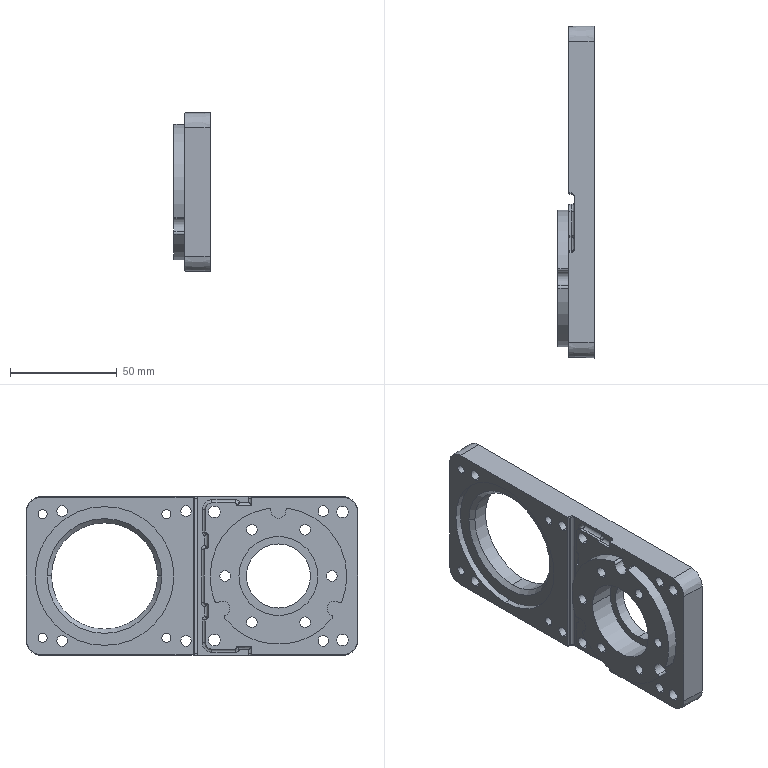Part | SolidWorks | features BaseBody 1 | 1 solid | 224 faces | box 17 x 155.419 x 74.419 mm | volume 93812 mm3 | cylinder 111 | plane 58 | cone 29 | spline 26 | commonest cylinder face diameters 1 x18 3 x18 4.98 x12 5 x12 2 x8 4.2 x8